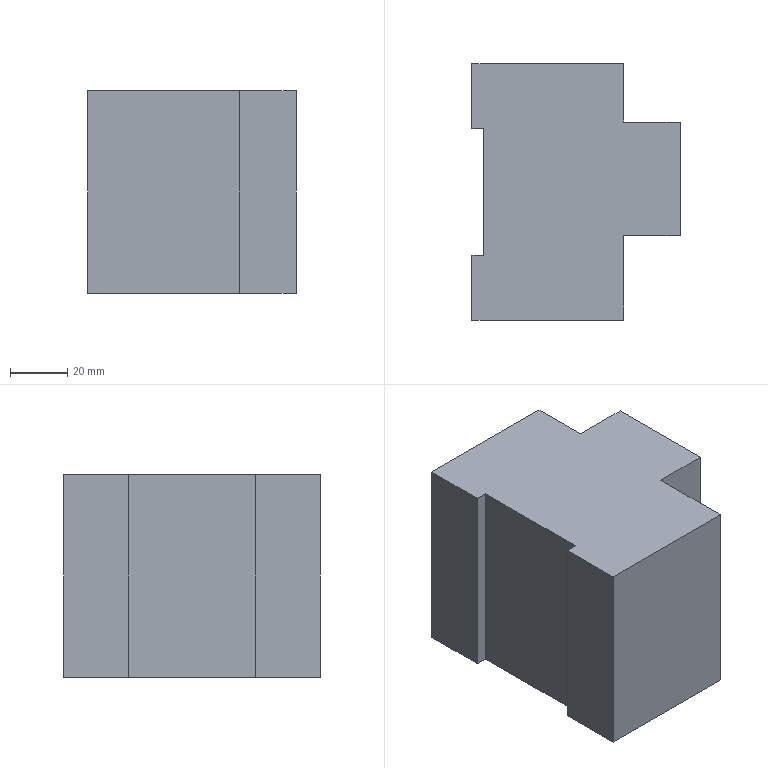Part | STEP file | Circuit breaker | 1 solid | 14 faces | box 73 x 90 x 71 mm | volume 383548 mm3 | plane 14
STEP:
#1=CARTESIAN_POINT('',(0.,0.,0.));
#2=DIRECTION('',(0.,0.,1.));
#3=DIRECTION('',(1.,0.,0.));
#4=AXIS2_PLACEMENT_3D('',#1,#2,#3);
#5=CARTESIAN_POINT('',(-36.5,45.,0.));
#6=VERTEX_POINT('',#5);
#7=CARTESIAN_POINT('',(-36.5,22.299,0.));
#8=VERTEX_POINT('',#7);
#9=CARTESIAN_POINT('',(-36.5,45.,0.));
#10=DIRECTION('',(0.,-1.,0.));
#11=VECTOR('',#10,1.);
#12=LINE('',#9,#11);
#13=CARTESIAN_POINT('',(-36.5,45.,71.));
#14=DIRECTION('',(1.,0.,0.));
#15=DIRECTION('',(0.,1.,0.));
#16=AXIS2_PLACEMENT_3D('',#13,#14,#15);
#17=PLANE('',#16);
#18=CARTESIAN_POINT('',(0.,-71.));
#19=DIRECTION('',(-1.,0.));
#20=VECTOR('',#19,1.);
#21=LINE('',#18,#20);
#22=(GEOMETRIC_REPRESENTATION_CONTEXT(2)PARAMETRIC_REPRESENTATION_CONTEXT()REPRESENTATION_CONTEXT('',''));
#23=DEFINITIONAL_REPRESENTATION('',(#21),#22);
#24=PCURVE('',#17,#23);
#25=CARTESIAN_POINT('',(0.,0.,0.));
#26=DIRECTION('',(0.,0.,-1.));
#27=DIRECTION('',(-1.,0.,0.));
#28=AXIS2_PLACEMENT_3D('',#25,#26,#27);
#29=PLANE('',#28);
#30=CARTESIAN_POINT('',(36.5,45.));
#31=DIRECTION('',(0.,-1.));
#32=VECTOR('',#31,1.);
#33=LINE('',#30,#32);
#34=(GEOMETRIC_REPRESENTATION_CONTEXT(2)PARAMETRIC_REPRESENTATION_CONTEXT()REPRESENTATION_CONTEXT('',''));
#35=DEFINITIONAL_REPRESENTATION('',(#33),#34);
#36=PCURVE('',#29,#35);
#37=SURFACE_CURVE('',#12,(#24,#36),.PCURVE_S1.);
#38=EDGE_CURVE('',#6,#8,#37,.T.);
#39=ORIENTED_EDGE('',*,*,#38,.T.);
#40=CARTESIAN_POINT('',(-36.5,22.299,71.));
#41=VERTEX_POINT('',#40);
#42=CARTESIAN_POINT('',(-36.5,22.299,0.));
#43=DIRECTION('',(0.,0.,1.));
#44=VECTOR('',#43,1.);
#45=LINE('',#42,#44);
#46=CARTESIAN_POINT('',(-22.701,-71.));
#47=DIRECTION('',(0.,1.));
#48=VECTOR('',#47,1.);
#49=LINE('',#46,#48);
#50=(GEOMETRIC_REPRESENTATION_CONTEXT(2)PARAMETRIC_REPRESENTATION_CONTEXT()REPRESENTATION_CONTEXT('',''));
#51=DEFINITIONAL_REPRESENTATION('',(#49),#50);
#52=PCURVE('',#17,#51);
#53=CARTESIAN_POINT('',(-36.5,22.299,0.));
#54=DIRECTION('',(0.,1.,0.));
#55=DIRECTION('',(0.,0.,1.));
#56=AXIS2_PLACEMENT_3D('',#53,#54,#55);
#57=PLANE('',#56);
#58=CARTESIAN_POINT('',(0.,0.));
#59=DIRECTION('',(1.,0.));
#60=VECTOR('',#59,1.);
#61=LINE('',#58,#60);
#62=(GEOMETRIC_REPRESENTATION_CONTEXT(2)PARAMETRIC_REPRESENTATION_CONTEXT()REPRESENTATION_CONTEXT('',''));
#63=DEFINITIONAL_REPRESENTATION('',(#61),#62);
#64=PCURVE('',#57,#63);
#65=SURFACE_CURVE('',#45,(#52,#64),.PCURVE_S1.);
#66=EDGE_CURVE('',#8,#41,#65,.T.);
#67=ORIENTED_EDGE('',*,*,#66,.T.);
#68=CARTESIAN_POINT('',(-36.5,45.,71.));
#69=VERTEX_POINT('',#68);
#70=CARTESIAN_POINT('',(-36.5,45.,71.));
#71=DIRECTION('',(0.,-1.,0.));
#72=VECTOR('',#71,1.);
#73=LINE('',#70,#72);
#74=CARTESIAN_POINT('',(0.,0.));
#75=DIRECTION('',(-1.,0.));
#76=VECTOR('',#75,1.);
#77=LINE('',#74,#76);
#78=(GEOMETRIC_REPRESENTATION_CONTEXT(2)PARAMETRIC_REPRESENTATION_CONTEXT()REPRESENTATION_CONTEXT('',''));
#79=DEFINITIONAL_REPRESENTATION('',(#77),#78);
#80=PCURVE('',#17,#79);
#81=CARTESIAN_POINT('',(0.,0.,71.));
#82=DIRECTION('',(0.,0.,-1.));
#83=DIRECTION('',(-1.,0.,0.));
#84=AXIS2_PLACEMENT_3D('',#81,#82,#83);
#85=PLANE('',#84);
#86=CARTESIAN_POINT('',(36.5,45.));
#87=DIRECTION('',(0.,-1.));
#88=VECTOR('',#87,1.);
#89=LINE('',#86,#88);
#90=(GEOMETRIC_REPRESENTATION_CONTEXT(2)PARAMETRIC_REPRESENTATION_CONTEXT()REPRESENTATION_CONTEXT('',''));
#91=DEFINITIONAL_REPRESENTATION('',(#89),#90);
#92=PCURVE('',#85,#91);
#93=SURFACE_CURVE('',#73,(#80,#92),.PCURVE_S1.);
#94=EDGE_CURVE('',#69,#41,#93,.T.);
#95=ORIENTED_EDGE('',*,*,#94,.F.);
#96=CARTESIAN_POINT('',(-36.5,45.,71.));
#97=DIRECTION('',(0.,0.,-1.));
#98=VECTOR('',#97,1.);
#99=LINE('',#96,#98);
#100=CARTESIAN_POINT('',(0.,0.));
#101=DIRECTION('',(0.,-1.));
#102=VECTOR('',#101,1.);
#103=LINE('',#100,#102);
#104=(GEOMETRIC_REPRESENTATION_CONTEXT(2)PARAMETRIC_REPRESENTATION_CONTEXT()REPRESENTATION_CONTEXT('',''));
#105=DEFINITIONAL_REPRESENTATION('',(#103),#104);
#106=PCURVE('',#17,#105);
#107=CARTESIAN_POINT('',(36.5,45.,71.));
#108=DIRECTION('',(0.,-1.,0.));
#109=DIRECTION('',(1.,0.,0.));
#110=AXIS2_PLACEMENT_3D('',#107,#108,#109);
#111=PLANE('',#110);
#112=CARTESIAN_POINT('',(-73.,0.));
#113=DIRECTION('',(0.,-1.));
#114=VECTOR('',#113,1.);
#115=LINE('',#112,#114);
#116=(GEOMETRIC_REPRESENTATION_CONTEXT(2)PARAMETRIC_REPRESENTATION_CONTEXT()REPRESENTATION_CONTEXT('',''));
#117=DEFINITIONAL_REPRESENTATION('',(#115),#116);
#118=PCURVE('',#111,#117);
#119=SURFACE_CURVE('',#99,(#106,#118),.PCURVE_S1.);
#120=EDGE_CURVE('',#69,#6,#119,.T.);
#121=ORIENTED_EDGE('',*,*,#120,.T.);
#122=EDGE_LOOP('',(#39,#67,#95,#121));
#123=FACE_BOUND('',#122,.T.);
#124=ADVANCED_FACE('',(#123),#17,.F.);
#125=CARTESIAN_POINT('',(-36.5,-22.299,71.));
#126=VERTEX_POINT('',#125);
#127=CARTESIAN_POINT('',(-36.5,-45.,71.));
#128=VERTEX_POINT('',#127);
#129=CARTESIAN_POINT('',(-36.5,45.,71.));
#130=DIRECTION('',(0.,-1.,0.));
#131=VECTOR('',#130,1.);
#132=LINE('',#129,#131);
#133=CARTESIAN_POINT('',(-36.5,45.,71.));
#134=DIRECTION('',(1.,0.,0.));
#135=DIRECTION('',(0.,1.,0.));
#136=AXIS2_PLACEMENT_3D('',#133,#134,#135);
#137=PLANE('',#136);
#138=CARTESIAN_POINT('',(0.,0.));
#139=DIRECTION('',(-1.,0.));
#140=VECTOR('',#139,1.);
#141=LINE('',#138,#140);
#142=(GEOMETRIC_REPRESENTATION_CONTEXT(2)PARAMETRIC_REPRESENTATION_CONTEXT()REPRESENTATION_CONTEXT('',''));
#143=DEFINITIONAL_REPRESENTATION('',(#141),#142);
#144=PCURVE('',#137,#143);
#145=CARTESIAN_POINT('',(36.5,45.));
#146=DIRECTION('',(0.,-1.));
#147=VECTOR('',#146,1.);
#148=LINE('',#145,#147);
#149=(GEOMETRIC_REPRESENTATION_CONTEXT(2)PARAMETRIC_REPRESENTATION_CONTEXT()REPRESENTATION_CONTEXT('',''));
#150=DEFINITIONAL_REPRESENTATION('',(#148),#149);
#151=PCURVE('',#85,#150);
#152=SURFACE_CURVE('',#132,(#144,#151),.PCURVE_S1.);
#153=EDGE_CURVE('',#126,#128,#152,.T.);
#154=ORIENTED_EDGE('',*,*,#153,.F.);
#155=CARTESIAN_POINT('',(-36.5,-22.299,0.));
#156=VERTEX_POINT('',#155);
#157=CARTESIAN_POINT('',(-36.5,-22.299,0.));
#158=DIRECTION('',(0.,0.,1.));
#159=VECTOR('',#158,1.);
#160=LINE('',#157,#159);
#161=CARTESIAN_POINT('',(-67.299,-71.));
#162=DIRECTION('',(0.,1.));
#163=VECTOR('',#162,1.);
#164=LINE('',#161,#163);
#165=(GEOMETRIC_REPRESENTATION_CONTEXT(2)PARAMETRIC_REPRESENTATION_CONTEXT()REPRESENTATION_CONTEXT('',''));
#166=DEFINITIONAL_REPRESENTATION('',(#164),#165);
#167=PCURVE('',#137,#166);
#168=CARTESIAN_POINT('',(-36.5,-22.299,0.));
#169=DIRECTION('',(0.,-1.,0.));
#170=DIRECTION('',(0.,0.,-1.));
#171=AXIS2_PLACEMENT_3D('',#168,#169,#170);
#172=PLANE('',#171);
#173=CARTESIAN_POINT('',(0.,0.));
#174=DIRECTION('',(-1.,0.));
#175=VECTOR('',#174,1.);
#176=LINE('',#173,#175);
#177=(GEOMETRIC_REPRESENTATION_CONTEXT(2)PARAMETRIC_REPRESENTATION_CONTEXT()REPRESENTATION_CONTEXT('',''));
#178=DEFINITIONAL_REPRESENTATION('',(#176),#177);
#179=PCURVE('',#172,#178);
#180=SURFACE_CURVE('',#160,(#167,#179),.PCURVE_S1.);
#181=EDGE_CURVE('',#156,#126,#180,.T.);
#182=ORIENTED_EDGE('',*,*,#181,.F.);
#183=CARTESIAN_POINT('',(-36.5,-45.,0.));
#184=VERTEX_POINT('',#183);
#185=CARTESIAN_POINT('',(-36.5,45.,0.));
#186=DIRECTION('',(0.,-1.,0.));
#187=VECTOR('',#186,1.);
#188=LINE('',#185,#187);
#189=CARTESIAN_POINT('',(0.,-71.));
#190=DIRECTION('',(-1.,0.));
#191=VECTOR('',#190,1.);
#192=LINE('',#189,#191);
#193=(GEOMETRIC_REPRESENTATION_CONTEXT(2)PARAMETRIC_REPRESENTATION_CONTEXT()REPRESENTATION_CONTEXT('',''));
#194=DEFINITIONAL_REPRESENTATION('',(#192),#193);
#195=PCURVE('',#137,#194);
#196=CARTESIAN_POINT('',(36.5,45.));
#197=DIRECTION('',(0.,-1.));
#198=VECTOR('',#197,1.);
#199=LINE('',#196,#198);
#200=(GEOMETRIC_REPRESENTATION_CONTEXT(2)PARAMETRIC_REPRESENTATION_CONTEXT()REPRESENTATION_CONTEXT('',''));
#201=DEFINITIONAL_REPRESENTATION('',(#199),#200);
#202=PCURVE('',#29,#201);
#203=SURFACE_CURVE('',#188,(#195,#202),.PCURVE_S1.);
#204=EDGE_CURVE('',#156,#184,#203,.T.);
#205=ORIENTED_EDGE('',*,*,#204,.T.);
#206=CARTESIAN_POINT('',(-36.5,-45.,71.));
#207=DIRECTION('',(0.,0.,-1.));
#208=VECTOR('',#207,1.);
#209=LINE('',#206,#208);
#210=CARTESIAN_POINT('',(-90.,0.));
#211=DIRECTION('',(0.,-1.));
#212=VECTOR('',#211,1.);
#213=LINE('',#210,#212);
#214=(GEOMETRIC_REPRESENTATION_CONTEXT(2)PARAMETRIC_REPRESENTATION_CONTEXT()REPRESENTATION_CONTEXT('',''));
#215=DEFINITIONAL_REPRESENTATION('',(#213),#214);
#216=PCURVE('',#137,#215);
#217=CARTESIAN_POINT('',(36.5,-45.,71.));
#218=DIRECTION('',(0.,1.,0.));
#219=DIRECTION('',(-1.,0.,0.));
#220=AXIS2_PLACEMENT_3D('',#217,#218,#219);
#221=PLANE('',#220);
#222=CARTESIAN_POINT('',(73.,0.));
#223=DIRECTION('',(0.,-1.));
#224=VECTOR('',#223,1.);
#225=LINE('',#222,#224);
#226=(GEOMETRIC_REPRESENTATION_CONTEXT(2)PARAMETRIC_REPRESENTATION_CONTEXT()REPRESENTATION_CONTEXT('',''));
#227=DEFINITIONAL_REPRESENTATION('',(#225),#226);
#228=PCURVE('',#221,#227);
#229=SURFACE_CURVE('',#209,(#216,#228),.PCURVE_S1.);
#230=EDGE_CURVE('',#128,#184,#229,.T.);
#231=ORIENTED_EDGE('',*,*,#230,.F.);
#232=EDGE_LOOP('',(#154,#182,#205,#231));
#233=FACE_BOUND('',#232,.T.);
#234=ADVANCED_FACE('',(#233),#137,.F.);
#235=CARTESIAN_POINT('',(16.786,-45.,0.));
#236=VERTEX_POINT('',#235);
#237=CARTESIAN_POINT('',(36.5,-45.,0.));
#238=DIRECTION('',(1.,0.,0.));
#239=VECTOR('',#238,1.);
#240=LINE('',#237,#239);
#241=CARTESIAN_POINT('',(0.,-71.));
#242=DIRECTION('',(-1.,0.));
#243=VECTOR('',#242,1.);
#244=LINE('',#241,#243);
#245=(GEOMETRIC_REPRESENTATION_CONTEXT(2)PARAMETRIC_REPRESENTATION_CONTEXT()REPRESENTATION_CONTEXT('',''));
#246=DEFINITIONAL_REPRESENTATION('',(#244),#245);
#247=PCURVE('',#221,#246);
#248=CARTESIAN_POINT('',(-36.5,-45.));
#249=DIRECTION('',(-1.,0.));
#250=VECTOR('',#249,1.);
#251=LINE('',#248,#250);
#252=(GEOMETRIC_REPRESENTATION_CONTEXT(2)PARAMETRIC_REPRESENTATION_CONTEXT()REPRESENTATION_CONTEXT('',''));
#253=DEFINITIONAL_REPRESENTATION('',(#251),#252);
#254=PCURVE('',#29,#253);
#255=SURFACE_CURVE('',#240,(#247,#254),.PCURVE_S1.);
#256=EDGE_CURVE('',#184,#236,#255,.T.);
#257=ORIENTED_EDGE('',*,*,#256,.T.);
#258=CARTESIAN_POINT('',(16.786,-45.,71.));
#259=VERTEX_POINT('',#258);
#260=CARTESIAN_POINT('',(16.786,-45.,0.));
#261=DIRECTION('',(0.,0.,1.));
#262=VECTOR('',#261,1.);
#263=LINE('',#260,#262);
#264=CARTESIAN_POINT('',(19.714,-71.));
#265=DIRECTION('',(0.,1.));
#266=VECTOR('',#265,1.);
#267=LINE('',#264,#266);
#268=(GEOMETRIC_REPRESENTATION_CONTEXT(2)PARAMETRIC_REPRESENTATION_CONTEXT()REPRESENTATION_CONTEXT('',''));
#269=DEFINITIONAL_REPRESENTATION('',(#267),#268);
#270=PCURVE('',#221,#269);
#271=CARTESIAN_POINT('',(16.786,-15.316,0.));
#272=DIRECTION('',(-1.,0.,0.));
#273=DIRECTION('',(0.,0.,1.));
#274=AXIS2_PLACEMENT_3D('',#271,#272,#273);
#275=PLANE('',#274);
#276=CARTESIAN_POINT('',(0.,-29.684));
#277=DIRECTION('',(1.,0.));
#278=VECTOR('',#277,1.);
#279=LINE('',#276,#278);
#280=(GEOMETRIC_REPRESENTATION_CONTEXT(2)PARAMETRIC_REPRESENTATION_CONTEXT()REPRESENTATION_CONTEXT('',''));
#281=DEFINITIONAL_REPRESENTATION('',(#279),#280);
#282=PCURVE('',#275,#281);
#283=SURFACE_CURVE('',#263,(#270,#282),.PCURVE_S1.);
#284=EDGE_CURVE('',#236,#259,#283,.T.);
#285=ORIENTED_EDGE('',*,*,#284,.T.);
#286=CARTESIAN_POINT('',(36.5,-45.,71.));
#287=DIRECTION('',(1.,0.,0.));
#288=VECTOR('',#287,1.);
#289=LINE('',#286,#288);
#290=CARTESIAN_POINT('',(0.,0.));
#291=DIRECTION('',(-1.,0.));
#292=VECTOR('',#291,1.);
#293=LINE('',#290,#292);
#294=(GEOMETRIC_REPRESENTATION_CONTEXT(2)PARAMETRIC_REPRESENTATION_CONTEXT()REPRESENTATION_CONTEXT('',''));
#295=DEFINITIONAL_REPRESENTATION('',(#293),#294);
#296=PCURVE('',#221,#295);
#297=CARTESIAN_POINT('',(-36.5,-45.));
#298=DIRECTION('',(-1.,0.));
#299=VECTOR('',#298,1.);
#300=LINE('',#297,#299);
#301=(GEOMETRIC_REPRESENTATION_CONTEXT(2)PARAMETRIC_REPRESENTATION_CONTEXT()REPRESENTATION_CONTEXT('',''));
#302=DEFINITIONAL_REPRESENTATION('',(#300),#301);
#303=PCURVE('',#85,#302);
#304=SURFACE_CURVE('',#289,(#296,#303),.PCURVE_S1.);
#305=EDGE_CURVE('',#128,#259,#304,.T.);
#306=ORIENTED_EDGE('',*,*,#305,.F.);
#307=ORIENTED_EDGE('',*,*,#230,.T.);
#308=EDGE_LOOP('',(#257,#285,#306,#307));
#309=FACE_BOUND('',#308,.T.);
#310=ADVANCED_FACE('',(#309),#221,.F.);
#311=CARTESIAN_POINT('',(36.5,-15.316,71.));
#312=VERTEX_POINT('',#311);
#313=CARTESIAN_POINT('',(36.5,24.49,71.));
#314=VERTEX_POINT('',#313);
#315=CARTESIAN_POINT('',(36.5,45.,71.));
#316=DIRECTION('',(0.,1.,0.));
#317=VECTOR('',#316,1.);
#318=LINE('',#315,#317);
#319=CARTESIAN_POINT('',(36.5,45.,71.));
#320=DIRECTION('',(-1.,0.,0.));
#321=DIRECTION('',(0.,-1.,0.));
#322=AXIS2_PLACEMENT_3D('',#319,#320,#321);
#323=PLANE('',#322);
#324=CARTESIAN_POINT('',(0.,0.));
#325=DIRECTION('',(-1.,0.));
#326=VECTOR('',#325,1.);
#327=LINE('',#324,#326);
#328=(GEOMETRIC_REPRESENTATION_CONTEXT(2)PARAMETRIC_REPRESENTATION_CONTEXT()REPRESENTATION_CONTEXT('',''));
#329=DEFINITIONAL_REPRESENTATION('',(#327),#328);
#330=PCURVE('',#323,#329);
#331=CARTESIAN_POINT('',(-36.5,45.));
#332=DIRECTION('',(0.,1.));
#333=VECTOR('',#332,1.);
#334=LINE('',#331,#333);
#335=(GEOMETRIC_REPRESENTATION_CONTEXT(2)PARAMETRIC_REPRESENTATION_CONTEXT()REPRESENTATION_CONTEXT('',''));
#336=DEFINITIONAL_REPRESENTATION('',(#334),#335);
#337=PCURVE('',#85,#336);
#338=SURFACE_CURVE('',#318,(#330,#337),.PCURVE_S1.);
#339=EDGE_CURVE('',#312,#314,#338,.T.);
#340=ORIENTED_EDGE('',*,*,#339,.F.);
#341=CARTESIAN_POINT('',(36.5,-15.316,0.));
#342=VERTEX_POINT('',#341);
#343=CARTESIAN_POINT('',(36.5,-15.316,0.));
#344=DIRECTION('',(0.,0.,1.));
#345=VECTOR('',#344,1.);
#346=LINE('',#343,#345);
#347=CARTESIAN_POINT('',(60.316,-71.));
#348=DIRECTION('',(0.,1.));
#349=VECTOR('',#348,1.);
#350=LINE('',#347,#349);
#351=(GEOMETRIC_REPRESENTATION_CONTEXT(2)PARAMETRIC_REPRESENTATION_CONTEXT()REPRESENTATION_CONTEXT('',''));
#352=DEFINITIONAL_REPRESENTATION('',(#350),#351);
#353=PCURVE('',#323,#352);
#354=CARTESIAN_POINT('',(36.5,-15.316,0.));
#355=DIRECTION('',(0.,1.,0.));
#356=DIRECTION('',(0.,0.,1.));
#357=AXIS2_PLACEMENT_3D('',#354,#355,#356);
#358=PLANE('',#357);
#359=CARTESIAN_POINT('',(0.,0.));
#360=DIRECTION('',(1.,0.));
#361=VECTOR('',#360,1.);
#362=LINE('',#359,#361);
#363=(GEOMETRIC_REPRESENTATION_CONTEXT(2)PARAMETRIC_REPRESENTATION_CONTEXT()REPRESENTATION_CONTEXT('',''));
#364=DEFINITIONAL_REPRESENTATION('',(#362),#363);
#365=PCURVE('',#358,#364);
#366=SURFACE_CURVE('',#346,(#353,#365),.PCURVE_S1.);
#367=EDGE_CURVE('',#342,#312,#366,.T.);
#368=ORIENTED_EDGE('',*,*,#367,.F.);
#369=CARTESIAN_POINT('',(36.5,24.49,0.));
#370=VERTEX_POINT('',#369);
#371=CARTESIAN_POINT('',(36.5,45.,0.));
#372=DIRECTION('',(0.,1.,0.));
#373=VECTOR('',#372,1.);
#374=LINE('',#371,#373);
#375=CARTESIAN_POINT('',(0.,-71.));
#376=DIRECTION('',(-1.,0.));
#377=VECTOR('',#376,1.);
#378=LINE('',#375,#377);
#379=(GEOMETRIC_REPRESENTATION_CONTEXT(2)PARAMETRIC_REPRESENTATION_CONTEXT()REPRESENTATION_CONTEXT('',''));
#380=DEFINITIONAL_REPRESENTATION('',(#378),#379);
#381=PCURVE('',#323,#380);
#382=CARTESIAN_POINT('',(-36.5,45.));
#383=DIRECTION('',(0.,1.));
#384=VECTOR('',#383,1.);
#385=LINE('',#382,#384);
#386=(GEOMETRIC_REPRESENTATION_CONTEXT(2)PARAMETRIC_REPRESENTATION_CONTEXT()REPRESENTATION_CONTEXT('',''));
#387=DEFINITIONAL_REPRESENTATION('',(#385),#386);
#388=PCURVE('',#29,#387);
#389=SURFACE_CURVE('',#374,(#381,#388),.PCURVE_S1.);
#390=EDGE_CURVE('',#342,#370,#389,.T.);
#391=ORIENTED_EDGE('',*,*,#390,.T.);
#392=CARTESIAN_POINT('',(36.5,24.49,0.));
#393=DIRECTION('',(0.,0.,1.));
#394=VECTOR('',#393,1.);
#395=LINE('',#392,#394);
#396=CARTESIAN_POINT('',(20.51,-71.));
#397=DIRECTION('',(0.,1.));
#398=VECTOR('',#397,1.);
#399=LINE('',#396,#398);
#400=(GEOMETRIC_REPRESENTATION_CONTEXT(2)PARAMETRIC_REPRESENTATION_CONTEXT()REPRESENTATION_CONTEXT('',''));
#401=DEFINITIONAL_REPRESENTATION('',(#399),#400);
#402=PCURVE('',#323,#401);
#403=CARTESIAN_POINT('',(16.786,24.49,0.));
#404=DIRECTION('',(0.,-1.,0.));
#405=DIRECTION('',(0.,0.,-1.));
#406=AXIS2_PLACEMENT_3D('',#403,#404,#405);
#407=PLANE('',#406);
#408=CARTESIAN_POINT('',(0.,19.714));
#409=DIRECTION('',(-1.,0.));
#410=VECTOR('',#409,1.);
#411=LINE('',#408,#410);
#412=(GEOMETRIC_REPRESENTATION_CONTEXT(2)PARAMETRIC_REPRESENTATION_CONTEXT()REPRESENTATION_CONTEXT('',''));
#413=DEFINITIONAL_REPRESENTATION('',(#411),#412);
#414=PCURVE('',#407,#413);
#415=SURFACE_CURVE('',#395,(#402,#414),.PCURVE_S1.);
#416=EDGE_CURVE('',#370,#314,#415,.T.);
#417=ORIENTED_EDGE('',*,*,#416,.T.);
#418=EDGE_LOOP('',(#340,#368,#391,#417));
#419=FACE_BOUND('',#418,.T.);
#420=ADVANCED_FACE('',(#419),#323,.F.);
#421=CARTESIAN_POINT('',(16.786,45.,71.));
#422=VERTEX_POINT('',#421);
#423=CARTESIAN_POINT('',(36.5,45.,71.));
#424=DIRECTION('',(-1.,0.,0.));
#425=VECTOR('',#424,1.);
#426=LINE('',#423,#425);
#427=CARTESIAN_POINT('',(0.,0.));
#428=DIRECTION('',(-1.,0.));
#429=VECTOR('',#428,1.);
#430=LINE('',#427,#429);
#431=(GEOMETRIC_REPRESENTATION_CONTEXT(2)PARAMETRIC_REPRESENTATION_CONTEXT()REPRESENTATION_CONTEXT('',''));
#432=DEFINITIONAL_REPRESENTATION('',(#430),#431);
#433=PCURVE('',#111,#432);
#434=CARTESIAN_POINT('',(-36.5,45.));
#435=DIRECTION('',(1.,0.));
#436=VECTOR('',#435,1.);
#437=LINE('',#434,#436);
#438=(GEOMETRIC_REPRESENTATION_CONTEXT(2)PARAMETRIC_REPRESENTATION_CONTEXT()REPRESENTATION_CONTEXT('',''));
#439=DEFINITIONAL_REPRESENTATION('',(#437),#438);
#440=PCURVE('',#85,#439);
#441=SURFACE_CURVE('',#426,(#433,#440),.PCURVE_S1.);
#442=EDGE_CURVE('',#422,#69,#441,.T.);
#443=ORIENTED_EDGE('',*,*,#442,.F.);
#444=CARTESIAN_POINT('',(16.786,45.,0.));
#445=VERTEX_POINT('',#444);
#446=CARTESIAN_POINT('',(16.786,45.,0.));
#447=DIRECTION('',(0.,0.,1.));
#448=VECTOR('',#447,1.);
#449=LINE('',#446,#448);
#450=CARTESIAN_POINT('',(-19.714,-71.));
#451=DIRECTION('',(0.,1.));
#452=VECTOR('',#451,1.);
#453=LINE('',#450,#452);
#454=(GEOMETRIC_REPRESENTATION_CONTEXT(2)PARAMETRIC_REPRESENTATION_CONTEXT()REPRESENTATION_CONTEXT('',''));
#455=DEFINITIONAL_REPRESENTATION('',(#453),#454);
#456=PCURVE('',#111,#455);
#457=CARTESIAN_POINT('',(16.786,45.,0.));
#458=DIRECTION('',(-1.,0.,0.));
#459=DIRECTION('',(0.,0.,1.));
#460=AXIS2_PLACEMENT_3D('',#457,#458,#459);
#461=PLANE('',#460);
#462=CARTESIAN_POINT('',(0.,0.));
#463=DIRECTION('',(1.,0.));
#464=VECTOR('',#463,1.);
#465=LINE('',#462,#464);
#466=(GEOMETRIC_REPRESENTATION_CONTEXT(2)PARAMETRIC_REPRESENTATION_CONTEXT()REPRESENTATION_CONTEXT('',''));
#467=DEFINITIONAL_REPRESENTATION('',(#465),#466);
#468=PCURVE('',#461,#467);
#469=SURFACE_CURVE('',#449,(#456,#468),.PCURVE_S1.);
#470=EDGE_CURVE('',#445,#422,#469,.T.);
#471=ORIENTED_EDGE('',*,*,#470,.F.);
#472=CARTESIAN_POINT('',(36.5,45.,0.));
#473=DIRECTION('',(-1.,0.,0.));
#474=VECTOR('',#473,1.);
#475=LINE('',#472,#474);
#476=CARTESIAN_POINT('',(0.,-71.));
#477=DIRECTION('',(-1.,0.));
#478=VECTOR('',#477,1.);
#479=LINE('',#476,#478);
#480=(GEOMETRIC_REPRESENTATION_CONTEXT(2)PARAMETRIC_REPRESENTATION_CONTEXT()REPRESENTATION_CONTEXT('',''));
#481=DEFINITIONAL_REPRESENTATION('',(#479),#480);
#482=PCURVE('',#111,#481);
#483=CARTESIAN_POINT('',(-36.5,45.));
#484=DIRECTION('',(1.,0.));
#485=VECTOR('',#484,1.);
#486=LINE('',#483,#485);
#487=(GEOMETRIC_REPRESENTATION_CONTEXT(2)PARAMETRIC_REPRESENTATION_CONTEXT()REPRESENTATION_CONTEXT('',''));
#488=DEFINITIONAL_REPRESENTATION('',(#486),#487);
#489=PCURVE('',#29,#488);
#490=SURFACE_CURVE('',#475,(#482,#489),.PCURVE_S1.);
#491=EDGE_CURVE('',#445,#6,#490,.T.);
#492=ORIENTED_EDGE('',*,*,#491,.T.);
#493=ORIENTED_EDGE('',*,*,#120,.F.);
#494=EDGE_LOOP('',(#443,#471,#492,#493));
#495=FACE_BOUND('',#494,.T.);
#496=ADVANCED_FACE('',(#495),#111,.F.);
#497=ORIENTED_EDGE('',*,*,#94,.T.);
#498=CARTESIAN_POINT('',(-32.5,22.299,71.));
#499=VERTEX_POINT('',#498);
#500=CARTESIAN_POINT('',(-36.5,22.299,71.));
#501=DIRECTION('',(-1.,0.,0.));
#502=VECTOR('',#501,1.);
#503=LINE('',#500,#502);
#504=CARTESIAN_POINT('',(36.5,22.299));
#505=DIRECTION('',(1.,0.));
#506=VECTOR('',#505,1.);
#507=LINE('',#504,#506);
#508=(GEOMETRIC_REPRESENTATION_CONTEXT(2)PARAMETRIC_REPRESENTATION_CONTEXT()REPRESENTATION_CONTEXT('',''));
#509=DEFINITIONAL_REPRESENTATION('',(#507),#508);
#510=PCURVE('',#85,#509);
#511=CARTESIAN_POINT('',(71.,0.));
#512=DIRECTION('',(0.,-1.));
#513=VECTOR('',#512,1.);
#514=LINE('',#511,#513);
#515=(GEOMETRIC_REPRESENTATION_CONTEXT(2)PARAMETRIC_REPRESENTATION_CONTEXT()REPRESENTATION_CONTEXT('',''));
#516=DEFINITIONAL_REPRESENTATION('',(#514),#515);
#517=PCURVE('',#57,#516);
#518=SURFACE_CURVE('',#503,(#510,#517),.PCURVE_S1.);
#519=EDGE_CURVE('',#499,#41,#518,.T.);
#520=ORIENTED_EDGE('',*,*,#519,.F.);
#521=CARTESIAN_POINT('',(-32.5,-22.299,71.));
#522=VERTEX_POINT('',#521);
#523=CARTESIAN_POINT('',(-32.5,22.299,71.));
#524=DIRECTION('',(0.,1.,0.));
#525=VECTOR('',#524,1.);
#526=LINE('',#523,#525);
#527=CARTESIAN_POINT('',(32.5,22.299));
#528=DIRECTION('',(0.,1.));
#529=VECTOR('',#528,1.);
#530=LINE('',#527,#529);
#531=(GEOMETRIC_REPRESENTATION_CONTEXT(2)PARAMETRIC_REPRESENTATION_CONTEXT()REPRESENTATION_CONTEXT('',''));
#532=DEFINITIONAL_REPRESENTATION('',(#530),#531);
#533=PCURVE('',#85,#532);
#534=CARTESIAN_POINT('',(-32.5,22.299,0.));
#535=DIRECTION('',(1.,0.,0.));
#536=DIRECTION('',(0.,0.,-1.));
#537=AXIS2_PLACEMENT_3D('',#534,#535,#536);
#538=PLANE('',#537);
#539=CARTESIAN_POINT('',(-71.,0.));
#540=DIRECTION('',(0.,1.));
#541=VECTOR('',#540,1.);
#542=LINE('',#539,#541);
#543=(GEOMETRIC_REPRESENTATION_CONTEXT(2)PARAMETRIC_REPRESENTATION_CONTEXT()REPRESENTATION_CONTEXT('',''));
#544=DEFINITIONAL_REPRESENTATION('',(#542),#543);
#545=PCURVE('',#538,#544);
#546=SURFACE_CURVE('',#526,(#533,#545),.PCURVE_S1.);
#547=EDGE_CURVE('',#522,#499,#546,.T.);
#548=ORIENTED_EDGE('',*,*,#547,.F.);
#549=CARTESIAN_POINT('',(-36.5,-22.299,71.));
#550=DIRECTION('',(1.,0.,0.));
#551=VECTOR('',#550,1.);
#552=LINE('',#549,#551);
#553=CARTESIAN_POINT('',(36.5,-22.299));
#554=DIRECTION('',(-1.,0.));
#555=VECTOR('',#554,1.);
#556=LINE('',#553,#555);
#557=(GEOMETRIC_REPRESENTATION_CONTEXT(2)PARAMETRIC_REPRESENTATION_CONTEXT()REPRESENTATION_CONTEXT('',''));
#558=DEFINITIONAL_REPRESENTATION('',(#556),#557);
#559=PCURVE('',#85,#558);
#560=CARTESIAN_POINT('',(-71.,0.));
#561=DIRECTION('',(0.,1.));
#562=VECTOR('',#561,1.);
#563=LINE('',#560,#562);
#564=(GEOMETRIC_REPRESENTATION_CONTEXT(2)PARAMETRIC_REPRESENTATION_CONTEXT()REPRESENTATION_CONTEXT('',''));
#565=DEFINITIONAL_REPRESENTATION('',(#563),#564);
#566=PCURVE('',#172,#565);
#567=SURFACE_CURVE('',#552,(#559,#566),.PCURVE_S1.);
#568=EDGE_CURVE('',#126,#522,#567,.T.);
#569=ORIENTED_EDGE('',*,*,#568,.F.);
#570=ORIENTED_EDGE('',*,*,#153,.T.);
#571=ORIENTED_EDGE('',*,*,#305,.T.);
#572=CARTESIAN_POINT('',(16.786,-15.316,71.));
#573=VERTEX_POINT('',#572);
#574=CARTESIAN_POINT('',(16.786,-15.316,71.));
#575=DIRECTION('',(0.,-1.,0.));
#576=VECTOR('',#575,1.);
#577=LINE('',#574,#576);
#578=CARTESIAN_POINT('',(-16.786,-15.316));
#579=DIRECTION('',(0.,-1.));
#580=VECTOR('',#579,1.);
#581=LINE('',#578,#580);
#582=(GEOMETRIC_REPRESENTATION_CONTEXT(2)PARAMETRIC_REPRESENTATION_CONTEXT()REPRESENTATION_CONTEXT('',''));
#583=DEFINITIONAL_REPRESENTATION('',(#581),#582);
#584=PCURVE('',#85,#583);
#585=CARTESIAN_POINT('',(71.,0.));
#586=DIRECTION('',(0.,-1.));
#587=VECTOR('',#586,1.);
#588=LINE('',#585,#587);
#589=(GEOMETRIC_REPRESENTATION_CONTEXT(2)PARAMETRIC_REPRESENTATION_CONTEXT()REPRESENTATION_CONTEXT('',''));
#590=DEFINITIONAL_REPRESENTATION('',(#588),#589);
#591=PCURVE('',#275,#590);
#592=SURFACE_CURVE('',#577,(#584,#591),.PCURVE_S1.);
#593=EDGE_CURVE('',#573,#259,#592,.T.);
#594=ORIENTED_EDGE('',*,*,#593,.F.);
#595=CARTESIAN_POINT('',(36.5,-15.316,71.));
#596=DIRECTION('',(-1.,0.,0.));
#597=VECTOR('',#596,1.);
#598=LINE('',#595,#597);
#599=CARTESIAN_POINT('',(-36.5,-15.316));
#600=DIRECTION('',(1.,0.));
#601=VECTOR('',#600,1.);
#602=LINE('',#599,#601);
#603=(GEOMETRIC_REPRESENTATION_CONTEXT(2)PARAMETRIC_REPRESENTATION_CONTEXT()REPRESENTATION_CONTEXT('',''));
#604=DEFINITIONAL_REPRESENTATION('',(#602),#603);
#605=PCURVE('',#85,#604);
#606=CARTESIAN_POINT('',(71.,0.));
#607=DIRECTION('',(0.,-1.));
#608=VECTOR('',#607,1.);
#609=LINE('',#606,#608);
#610=(GEOMETRIC_REPRESENTATION_CONTEXT(2)PARAMETRIC_REPRESENTATION_CONTEXT()REPRESENTATION_CONTEXT('',''));
#611=DEFINITIONAL_REPRESENTATION('',(#609),#610);
#612=PCURVE('',#358,#611);
#613=SURFACE_CURVE('',#598,(#605,#612),.PCURVE_S1.);
#614=EDGE_CURVE('',#312,#573,#613,.T.);
#615=ORIENTED_EDGE('',*,*,#614,.F.);
#616=ORIENTED_EDGE('',*,*,#339,.T.);
#617=CARTESIAN_POINT('',(16.786,24.49,71.));
#618=VERTEX_POINT('',#617);
#619=CARTESIAN_POINT('',(16.786,24.49,71.));
#620=DIRECTION('',(1.,0.,0.));
#621=VECTOR('',#620,1.);
#622=LINE('',#619,#621);
#623=CARTESIAN_POINT('',(-16.786,24.49));
#624=DIRECTION('',(-1.,0.));
#625=VECTOR('',#624,1.);
#626=LINE('',#623,#625);
#627=(GEOMETRIC_REPRESENTATION_CONTEXT(2)PARAMETRIC_REPRESENTATION_CONTEXT()REPRESENTATION_CONTEXT('',''));
#628=DEFINITIONAL_REPRESENTATION('',(#626),#627);
#629=PCURVE('',#85,#628);
#630=CARTESIAN_POINT('',(-71.,0.));
#631=DIRECTION('',(0.,1.));
#632=VECTOR('',#631,1.);
#633=LINE('',#630,#632);
#634=(GEOMETRIC_REPRESENTATION_CONTEXT(2)PARAMETRIC_REPRESENTATION_CONTEXT()REPRESENTATION_CONTEXT('',''));
#635=DEFINITIONAL_REPRESENTATION('',(#633),#634);
#636=PCURVE('',#407,#635);
#637=SURFACE_CURVE('',#622,(#629,#636),.PCURVE_S1.);
#638=EDGE_CURVE('',#618,#314,#637,.T.);
#639=ORIENTED_EDGE('',*,*,#638,.F.);
#640=CARTESIAN_POINT('',(16.786,45.,71.));
#641=DIRECTION('',(0.,-1.,0.));
#642=VECTOR('',#641,1.);
#643=LINE('',#640,#642);
#644=CARTESIAN_POINT('',(-16.786,45.));
#645=DIRECTION('',(0.,-1.));
#646=VECTOR('',#645,1.);
#647=LINE('',#644,#646);
#648=(GEOMETRIC_REPRESENTATION_CONTEXT(2)PARAMETRIC_REPRESENTATION_CONTEXT()REPRESENTATION_CONTEXT('',''));
#649=DEFINITIONAL_REPRESENTATION('',(#647),#648);
#650=PCURVE('',#85,#649);
#651=CARTESIAN_POINT('',(71.,0.));
#652=DIRECTION('',(0.,-1.));
#653=VECTOR('',#652,1.);
#654=LINE('',#651,#653);
#655=(GEOMETRIC_REPRESENTATION_CONTEXT(2)PARAMETRIC_REPRESENTATION_CONTEXT()REPRESENTATION_CONTEXT('',''));
#656=DEFINITIONAL_REPRESENTATION('',(#654),#655);
#657=PCURVE('',#461,#656);
#658=SURFACE_CURVE('',#643,(#650,#657),.PCURVE_S1.);
#659=EDGE_CURVE('',#422,#618,#658,.T.);
#660=ORIENTED_EDGE('',*,*,#659,.F.);
#661=ORIENTED_EDGE('',*,*,#442,.T.);
#662=EDGE_LOOP('',(#497,#520,#548,#569,#570,#571,#594,#615,#616,#639,#660,#661));
#663=FACE_BOUND('',#662,.T.);
#664=ADVANCED_FACE('',(#663),#85,.F.);
#665=CARTESIAN_POINT('',(-32.5,22.299,0.));
#666=VERTEX_POINT('',#665);
#667=CARTESIAN_POINT('',(-36.5,22.299,0.));
#668=DIRECTION('',(-1.,0.,0.));
#669=VECTOR('',#668,1.);
#670=LINE('',#667,#669);
#671=CARTESIAN_POINT('',(36.5,22.299));
#672=DIRECTION('',(1.,0.));
#673=VECTOR('',#672,1.);
#674=LINE('',#671,#673);
#675=(GEOMETRIC_REPRESENTATION_CONTEXT(2)PARAMETRIC_REPRESENTATION_CONTEXT()REPRESENTATION_CONTEXT('',''));
#676=DEFINITIONAL_REPRESENTATION('',(#674),#675);
#677=PCURVE('',#29,#676);
#678=CARTESIAN_POINT('',(0.,0.));
#679=DIRECTION('',(0.,-1.));
#680=VECTOR('',#679,1.);
#681=LINE('',#678,#680);
#682=(GEOMETRIC_REPRESENTATION_CONTEXT(2)PARAMETRIC_REPRESENTATION_CONTEXT()REPRESENTATION_CONTEXT('',''));
#683=DEFINITIONAL_REPRESENTATION('',(#681),#682);
#684=PCURVE('',#57,#683);
#685=SURFACE_CURVE('',#670,(#677,#684),.PCURVE_S1.);
#686=EDGE_CURVE('',#666,#8,#685,.T.);
#687=ORIENTED_EDGE('',*,*,#686,.T.);
#688=ORIENTED_EDGE('',*,*,#38,.F.);
#689=ORIENTED_EDGE('',*,*,#491,.F.);
#690=CARTESIAN_POINT('',(16.786,24.49,0.));
#691=VERTEX_POINT('',#690);
#692=CARTESIAN_POINT('',(16.786,45.,0.));
#693=DIRECTION('',(0.,-1.,0.));
#694=VECTOR('',#693,1.);
#695=LINE('',#692,#694);
#696=CARTESIAN_POINT('',(-16.786,45.));
#697=DIRECTION('',(0.,-1.));
#698=VECTOR('',#697,1.);
#699=LINE('',#696,#698);
#700=(GEOMETRIC_REPRESENTATION_CONTEXT(2)PARAMETRIC_REPRESENTATION_CONTEXT()REPRESENTATION_CONTEXT('',''));
#701=DEFINITIONAL_REPRESENTATION('',(#699),#700);
#702=PCURVE('',#29,#701);
#703=CARTESIAN_POINT('',(0.,0.));
#704=DIRECTION('',(0.,-1.));
#705=VECTOR('',#704,1.);
#706=LINE('',#703,#705);
#707=(GEOMETRIC_REPRESENTATION_CONTEXT(2)PARAMETRIC_REPRESENTATION_CONTEXT()REPRESENTATION_CONTEXT('',''));
#708=DEFINITIONAL_REPRESENTATION('',(#706),#707);
#709=PCURVE('',#461,#708);
#710=SURFACE_CURVE('',#695,(#702,#709),.PCURVE_S1.);
#711=EDGE_CURVE('',#445,#691,#710,.T.);
#712=ORIENTED_EDGE('',*,*,#711,.T.);
#713=CARTESIAN_POINT('',(16.786,24.49,0.));
#714=DIRECTION('',(1.,0.,0.));
#715=VECTOR('',#714,1.);
#716=LINE('',#713,#715);
#717=CARTESIAN_POINT('',(-16.786,24.49));
#718=DIRECTION('',(-1.,0.));
#719=VECTOR('',#718,1.);
#720=LINE('',#717,#719);
#721=(GEOMETRIC_REPRESENTATION_CONTEXT(2)PARAMETRIC_REPRESENTATION_CONTEXT()REPRESENTATION_CONTEXT('',''));
#722=DEFINITIONAL_REPRESENTATION('',(#720),#721);
#723=PCURVE('',#29,#722);
#724=CARTESIAN_POINT('',(0.,0.));
#725=DIRECTION('',(0.,1.));
#726=VECTOR('',#725,1.);
#727=LINE('',#724,#726);
#728=(GEOMETRIC_REPRESENTATION_CONTEXT(2)PARAMETRIC_REPRESENTATION_CONTEXT()REPRESENTATION_CONTEXT('',''));
#729=DEFINITIONAL_REPRESENTATION('',(#727),#728);
#730=PCURVE('',#407,#729);
#731=SURFACE_CURVE('',#716,(#723,#730),.PCURVE_S1.);
#732=EDGE_CURVE('',#691,#370,#731,.T.);
#733=ORIENTED_EDGE('',*,*,#732,.T.);
#734=ORIENTED_EDGE('',*,*,#390,.F.);
#735=CARTESIAN_POINT('',(16.786,-15.316,0.));
#736=VERTEX_POINT('',#735);
#737=CARTESIAN_POINT('',(36.5,-15.316,0.));
#738=DIRECTION('',(-1.,0.,0.));
#739=VECTOR('',#738,1.);
#740=LINE('',#737,#739);
#741=CARTESIAN_POINT('',(-36.5,-15.316));
#742=DIRECTION('',(1.,0.));
#743=VECTOR('',#742,1.);
#744=LINE('',#741,#743);
#745=(GEOMETRIC_REPRESENTATION_CONTEXT(2)PARAMETRIC_REPRESENTATION_CONTEXT()REPRESENTATION_CONTEXT('',''));
#746=DEFINITIONAL_REPRESENTATION('',(#744),#745);
#747=PCURVE('',#29,#746);
#748=CARTESIAN_POINT('',(0.,0.));
#749=DIRECTION('',(0.,-1.));
#750=VECTOR('',#749,1.);
#751=LINE('',#748,#750);
#752=(GEOMETRIC_REPRESENTATION_CONTEXT(2)PARAMETRIC_REPRESENTATION_CONTEXT()REPRESENTATION_CONTEXT('',''));
#753=DEFINITIONAL_REPRESENTATION('',(#751),#752);
#754=PCURVE('',#358,#753);
#755=SURFACE_CURVE('',#740,(#747,#754),.PCURVE_S1.);
#756=EDGE_CURVE('',#342,#736,#755,.T.);
#757=ORIENTED_EDGE('',*,*,#756,.T.);
#758=CARTESIAN_POINT('',(16.786,-15.316,0.));
#759=DIRECTION('',(0.,-1.,0.));
#760=VECTOR('',#759,1.);
#761=LINE('',#758,#760);
#762=CARTESIAN_POINT('',(-16.786,-15.316));
#763=DIRECTION('',(0.,-1.));
#764=VECTOR('',#763,1.);
#765=LINE('',#762,#764);
#766=(GEOMETRIC_REPRESENTATION_CONTEXT(2)PARAMETRIC_REPRESENTATION_CONTEXT()REPRESENTATION_CONTEXT('',''));
#767=DEFINITIONAL_REPRESENTATION('',(#765),#766);
#768=PCURVE('',#29,#767);
#769=CARTESIAN_POINT('',(0.,0.));
#770=DIRECTION('',(0.,-1.));
#771=VECTOR('',#770,1.);
#772=LINE('',#769,#771);
#773=(GEOMETRIC_REPRESENTATION_CONTEXT(2)PARAMETRIC_REPRESENTATION_CONTEXT()REPRESENTATION_CONTEXT('',''));
#774=DEFINITIONAL_REPRESENTATION('',(#772),#773);
#775=PCURVE('',#275,#774);
#776=SURFACE_CURVE('',#761,(#768,#775),.PCURVE_S1.);
#777=EDGE_CURVE('',#736,#236,#776,.T.);
#778=ORIENTED_EDGE('',*,*,#777,.T.);
#779=ORIENTED_EDGE('',*,*,#256,.F.);
#780=ORIENTED_EDGE('',*,*,#204,.F.);
#781=CARTESIAN_POINT('',(-32.5,-22.299,0.));
#782=VERTEX_POINT('',#781);
#783=CARTESIAN_POINT('',(-36.5,-22.299,0.));
#784=DIRECTION('',(1.,0.,0.));
#785=VECTOR('',#784,1.);
#786=LINE('',#783,#785);
#787=CARTESIAN_POINT('',(36.5,-22.299));
#788=DIRECTION('',(-1.,0.));
#789=VECTOR('',#788,1.);
#790=LINE('',#787,#789);
#791=(GEOMETRIC_REPRESENTATION_CONTEXT(2)PARAMETRIC_REPRESENTATION_CONTEXT()REPRESENTATION_CONTEXT('',''));
#792=DEFINITIONAL_REPRESENTATION('',(#790),#791);
#793=PCURVE('',#29,#792);
#794=CARTESIAN_POINT('',(0.,0.));
#795=DIRECTION('',(0.,1.));
#796=VECTOR('',#795,1.);
#797=LINE('',#794,#796);
#798=(GEOMETRIC_REPRESENTATION_CONTEXT(2)PARAMETRIC_REPRESENTATION_CONTEXT()REPRESENTATION_CONTEXT('',''));
#799=DEFINITIONAL_REPRESENTATION('',(#797),#798);
#800=PCURVE('',#172,#799);
#801=SURFACE_CURVE('',#786,(#793,#800),.PCURVE_S1.);
#802=EDGE_CURVE('',#156,#782,#801,.T.);
#803=ORIENTED_EDGE('',*,*,#802,.T.);
#804=CARTESIAN_POINT('',(-32.5,22.299,0.));
#805=DIRECTION('',(0.,1.,0.));
#806=VECTOR('',#805,1.);
#807=LINE('',#804,#806);
#808=CARTESIAN_POINT('',(32.5,22.299));
#809=DIRECTION('',(0.,1.));
#810=VECTOR('',#809,1.);
#811=LINE('',#808,#810);
#812=(GEOMETRIC_REPRESENTATION_CONTEXT(2)PARAMETRIC_REPRESENTATION_CONTEXT()REPRESENTATION_CONTEXT('',''));
#813=DEFINITIONAL_REPRESENTATION('',(#811),#812);
#814=PCURVE('',#29,#813);
#815=CARTESIAN_POINT('',(0.,0.));
#816=DIRECTION('',(0.,1.));
#817=VECTOR('',#816,1.);
#818=LINE('',#815,#817);
#819=(GEOMETRIC_REPRESENTATION_CONTEXT(2)PARAMETRIC_REPRESENTATION_CONTEXT()REPRESENTATION_CONTEXT('',''));
#820=DEFINITIONAL_REPRESENTATION('',(#818),#819);
#821=PCURVE('',#538,#820);
#822=SURFACE_CURVE('',#807,(#814,#821),.PCURVE_S1.);
#823=EDGE_CURVE('',#782,#666,#822,.T.);
#824=ORIENTED_EDGE('',*,*,#823,.T.);
#825=EDGE_LOOP('',(#687,#688,#689,#712,#733,#734,#757,#778,#779,#780,#803,#824));
#826=FACE_BOUND('',#825,.T.);
#827=ADVANCED_FACE('',(#826),#29,.T.);
#828=ORIENTED_EDGE('',*,*,#659,.T.);
#829=CARTESIAN_POINT('',(16.786,24.49,0.));
#830=DIRECTION('',(0.,0.,1.));
#831=VECTOR('',#830,1.);
#832=LINE('',#829,#831);
#833=CARTESIAN_POINT('',(0.,-20.51));
#834=DIRECTION('',(1.,0.));
#835=VECTOR('',#834,1.);
#836=LINE('',#833,#835);
#837=(GEOMETRIC_REPRESENTATION_CONTEXT(2)PARAMETRIC_REPRESENTATION_CONTEXT()REPRESENTATION_CONTEXT('',''));
#838=DEFINITIONAL_REPRESENTATION('',(#836),#837);
#839=PCURVE('',#461,#838);
#840=CARTESIAN_POINT('',(0.,0.));
#841=DIRECTION('',(-1.,0.));
#842=VECTOR('',#841,1.);
#843=LINE('',#840,#842);
#844=(GEOMETRIC_REPRESENTATION_CONTEXT(2)PARAMETRIC_REPRESENTATION_CONTEXT()REPRESENTATION_CONTEXT('',''));
#845=DEFINITIONAL_REPRESENTATION('',(#843),#844);
#846=PCURVE('',#407,#845);
#847=SURFACE_CURVE('',#832,(#839,#846),.PCURVE_S1.);
#848=EDGE_CURVE('',#691,#618,#847,.T.);
#849=ORIENTED_EDGE('',*,*,#848,.F.);
#850=ORIENTED_EDGE('',*,*,#711,.F.);
#851=ORIENTED_EDGE('',*,*,#470,.T.);
#852=EDGE_LOOP('',(#828,#849,#850,#851));
#853=FACE_BOUND('',#852,.T.);
#854=ADVANCED_FACE('',(#853),#461,.F.);
#855=ORIENTED_EDGE('',*,*,#638,.T.);
#856=ORIENTED_EDGE('',*,*,#416,.F.);
#857=ORIENTED_EDGE('',*,*,#732,.F.);
#858=ORIENTED_EDGE('',*,*,#848,.T.);
#859=EDGE_LOOP('',(#855,#856,#857,#858));
#860=FACE_BOUND('',#859,.T.);
#861=ADVANCED_FACE('',(#860),#407,.F.);
#862=ORIENTED_EDGE('',*,*,#593,.T.);
#863=ORIENTED_EDGE('',*,*,#284,.F.);
#864=ORIENTED_EDGE('',*,*,#777,.F.);
#865=CARTESIAN_POINT('',(16.786,-15.316,0.));
#866=DIRECTION('',(0.,0.,1.));
#867=VECTOR('',#866,1.);
#868=LINE('',#865,#867);
#869=CARTESIAN_POINT('',(0.,0.));
#870=DIRECTION('',(1.,0.));
#871=VECTOR('',#870,1.);
#872=LINE('',#869,#871);
#873=(GEOMETRIC_REPRESENTATION_CONTEXT(2)PARAMETRIC_REPRESENTATION_CONTEXT()REPRESENTATION_CONTEXT('',''));
#874=DEFINITIONAL_REPRESENTATION('',(#872),#873);
#875=PCURVE('',#275,#874);
#876=CARTESIAN_POINT('',(0.,-19.714));
#877=DIRECTION('',(1.,0.));
#878=VECTOR('',#877,1.);
#879=LINE('',#876,#878);
#880=(GEOMETRIC_REPRESENTATION_CONTEXT(2)PARAMETRIC_REPRESENTATION_CONTEXT()REPRESENTATION_CONTEXT('',''));
#881=DEFINITIONAL_REPRESENTATION('',(#879),#880);
#882=PCURVE('',#358,#881);
#883=SURFACE_CURVE('',#868,(#875,#882),.PCURVE_S1.);
#884=EDGE_CURVE('',#736,#573,#883,.T.);
#885=ORIENTED_EDGE('',*,*,#884,.T.);
#886=EDGE_LOOP('',(#862,#863,#864,#885));
#887=FACE_BOUND('',#886,.T.);
#888=ADVANCED_FACE('',(#887),#275,.F.);
#889=ORIENTED_EDGE('',*,*,#614,.T.);
#890=ORIENTED_EDGE('',*,*,#884,.F.);
#891=ORIENTED_EDGE('',*,*,#756,.F.);
#892=ORIENTED_EDGE('',*,*,#367,.T.);
#893=EDGE_LOOP('',(#889,#890,#891,#892));
#894=FACE_BOUND('',#893,.T.);
#895=ADVANCED_FACE('',(#894),#358,.F.);
#896=ORIENTED_EDGE('',*,*,#519,.T.);
#897=ORIENTED_EDGE('',*,*,#66,.F.);
#898=ORIENTED_EDGE('',*,*,#686,.F.);
#899=CARTESIAN_POINT('',(-32.5,22.299,0.));
#900=DIRECTION('',(0.,0.,1.));
#901=VECTOR('',#900,1.);
#902=LINE('',#899,#901);
#903=CARTESIAN_POINT('',(0.,4.));
#904=DIRECTION('',(1.,0.));
#905=VECTOR('',#904,1.);
#906=LINE('',#903,#905);
#907=(GEOMETRIC_REPRESENTATION_CONTEXT(2)PARAMETRIC_REPRESENTATION_CONTEXT()REPRESENTATION_CONTEXT('',''));
#908=DEFINITIONAL_REPRESENTATION('',(#906),#907);
#909=PCURVE('',#57,#908);
#910=CARTESIAN_POINT('',(0.,0.));
#911=DIRECTION('',(-1.,0.));
#912=VECTOR('',#911,1.);
#913=LINE('',#910,#912);
#914=(GEOMETRIC_REPRESENTATION_CONTEXT(2)PARAMETRIC_REPRESENTATION_CONTEXT()REPRESENTATION_CONTEXT('',''));
#915=DEFINITIONAL_REPRESENTATION('',(#913),#914);
#916=PCURVE('',#538,#915);
#917=SURFACE_CURVE('',#902,(#909,#916),.PCURVE_S1.);
#918=EDGE_CURVE('',#666,#499,#917,.T.);
#919=ORIENTED_EDGE('',*,*,#918,.T.);
#920=EDGE_LOOP('',(#896,#897,#898,#919));
#921=FACE_BOUND('',#920,.T.);
#922=ADVANCED_FACE('',(#921),#57,.F.);
#923=ORIENTED_EDGE('',*,*,#547,.T.);
#924=ORIENTED_EDGE('',*,*,#918,.F.);
#925=ORIENTED_EDGE('',*,*,#823,.F.);
#926=CARTESIAN_POINT('',(-32.5,-22.299,0.));
#927=DIRECTION('',(0.,0.,1.));
#928=VECTOR('',#927,1.);
#929=LINE('',#926,#928);
#930=CARTESIAN_POINT('',(0.,-44.597));
#931=DIRECTION('',(-1.,0.));
#932=VECTOR('',#931,1.);
#933=LINE('',#930,#932);
#934=(GEOMETRIC_REPRESENTATION_CONTEXT(2)PARAMETRIC_REPRESENTATION_CONTEXT()REPRESENTATION_CONTEXT('',''));
#935=DEFINITIONAL_REPRESENTATION('',(#933),#934);
#936=PCURVE('',#538,#935);
#937=CARTESIAN_POINT('',(0.,4.));
#938=DIRECTION('',(-1.,0.));
#939=VECTOR('',#938,1.);
#940=LINE('',#937,#939);
#941=(GEOMETRIC_REPRESENTATION_CONTEXT(2)PARAMETRIC_REPRESENTATION_CONTEXT()REPRESENTATION_CONTEXT('',''));
#942=DEFINITIONAL_REPRESENTATION('',(#940),#941);
#943=PCURVE('',#172,#942);
#944=SURFACE_CURVE('',#929,(#936,#943),.PCURVE_S1.);
#945=EDGE_CURVE('',#782,#522,#944,.T.);
#946=ORIENTED_EDGE('',*,*,#945,.T.);
#947=EDGE_LOOP('',(#923,#924,#925,#946));
#948=FACE_BOUND('',#947,.T.);
#949=ADVANCED_FACE('',(#948),#538,.F.);
#950=ORIENTED_EDGE('',*,*,#568,.T.);
#951=ORIENTED_EDGE('',*,*,#945,.F.);
#952=ORIENTED_EDGE('',*,*,#802,.F.);
#953=ORIENTED_EDGE('',*,*,#181,.T.);
#954=EDGE_LOOP('',(#950,#951,#952,#953));
#955=FACE_BOUND('',#954,.T.);
#956=ADVANCED_FACE('',(#955),#172,.F.);
#957=CLOSED_SHELL('',(#124,#234,#310,#420,#496,#664,#827,#854,#861,#888,#895,#922,#949,#956));
#958=MANIFOLD_SOLID_BREP('',#957);
#959=(LENGTH_UNIT()NAMED_UNIT(*)SI_UNIT(.MILLI.,.METRE.));
#960=UNCERTAINTY_MEASURE_WITH_UNIT(LENGTH_MEASURE(0.0000001),#959,'','');
#961=(NAMED_UNIT(*)PLANE_ANGLE_UNIT()SI_UNIT($,.RADIAN.));
#962=(NAMED_UNIT(*)SI_UNIT($,.STERADIAN.)SOLID_ANGLE_UNIT());
#963=(GEOMETRIC_REPRESENTATION_CONTEXT(3)GLOBAL_UNCERTAINTY_ASSIGNED_CONTEXT((#960))GLOBAL_UNIT_ASSIGNED_CONTEXT((#959,#961,#962))REPRESENTATION_CONTEXT('',''));
#964=ADVANCED_BREP_SHAPE_REPRESENTATION('',(#4,#958),#963);